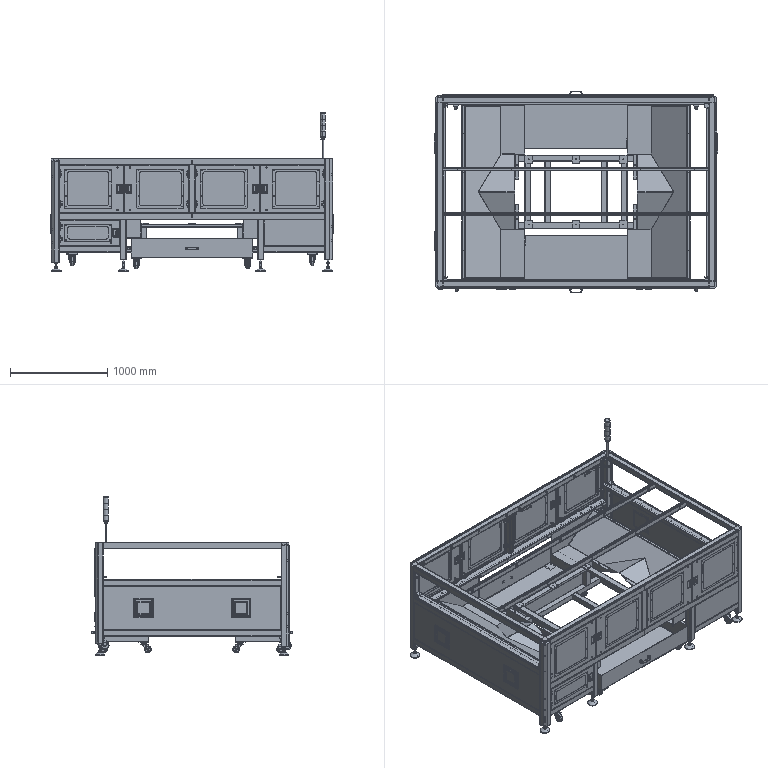Part | SolidWorks | features CompositeCurve 5, ReferencePattern 4, LocalLPattern 1 | 532 solids | 12783 faces | volume 89338303 mm3 | plane 6867 | cylinder 5004 | spline 354 | cone 318 | torus 216 | sphere 24 | commonest cylinder face diameters 7 x1058 5 x672 6 x624 4 x498 10 x358 12 x220